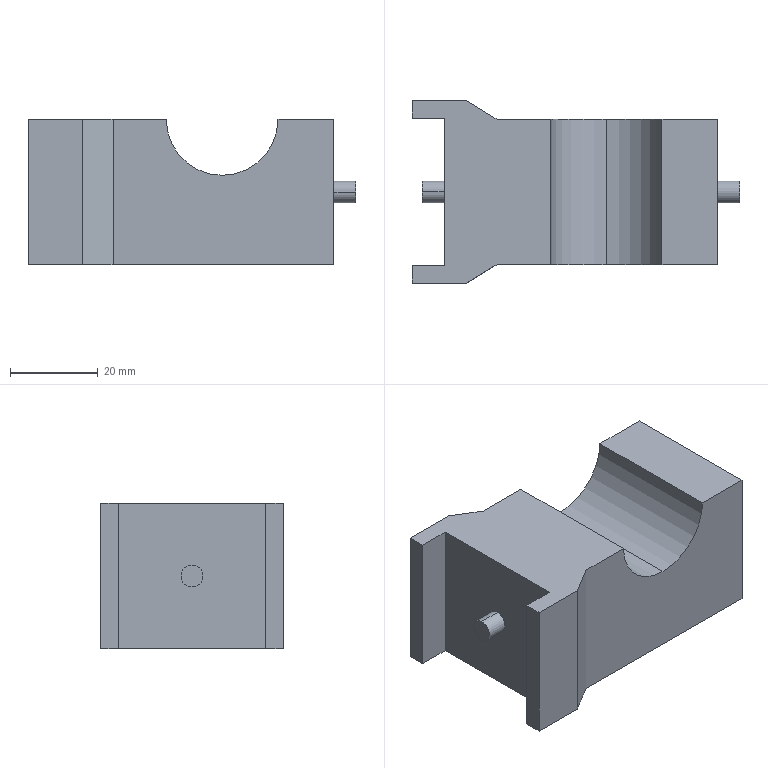Part | SolidWorks | features BaseBody 1, ICE 1 | 1 solid | 23 faces | box 74.5 x 41.5 x 33 mm | volume 63883 mm3 | plane 17 | cylinder 6 | commonest cylinder face diameters 5 x4 25.4 x2
STEP:
#1=CARTESIAN_POINT('',(12.4,16.5,16.5));
#2=VERTEX_POINT('',#1);
#3=CARTESIAN_POINT('',(-0.3,16.5,3.8));
#4=VERTEX_POINT('',#3);
#5=CARTESIAN_POINT('',(-0.3,16.5,16.5));
#6=DIRECTION('',(0.,1.,0.));
#7=DIRECTION('',(1.,0.,0.));
#8=AXIS2_PLACEMENT_3D('',#5,#6,#7);
#9=CIRCLE('',#8,12.7);
#10=EDGE_CURVE('',#2,#4,#9,.T.);
#11=ORIENTED_EDGE('',*,*,#10,.T.);
#12=CARTESIAN_POINT('',(-0.3,-16.5,3.8));
#13=VERTEX_POINT('',#12);
#14=CARTESIAN_POINT('',(-0.3,20.75,3.8));
#15=DIRECTION('',(0.,-1.,0.));
#16=VECTOR('',#15,1000.);
#17=LINE('',#14,#16);
#18=EDGE_CURVE('',#4,#13,#17,.T.);
#19=ORIENTED_EDGE('',*,*,#18,.T.);
#20=CARTESIAN_POINT('',(12.4,-16.5,16.5));
#21=VERTEX_POINT('',#20);
#22=CARTESIAN_POINT('',(-0.3,-16.5,16.5));
#23=DIRECTION('',(0.,-1.,0.));
#24=DIRECTION('',(0.,0.,1.));
#25=AXIS2_PLACEMENT_3D('',#22,#23,#24);
#26=CIRCLE('',#25,12.7);
#27=EDGE_CURVE('',#13,#21,#26,.T.);
#28=ORIENTED_EDGE('',*,*,#27,.T.);
#29=CARTESIAN_POINT('',(12.4,20.75,16.5));
#30=DIRECTION('',(0.,1.,0.));
#31=VECTOR('',#30,1000.);
#32=LINE('',#29,#31);
#33=EDGE_CURVE('',#21,#2,#32,.T.);
#34=ORIENTED_EDGE('',*,*,#33,.T.);
#35=EDGE_LOOP('',(#11,#19,#28,#34));
#36=FACE_OUTER_BOUND('',#35,.T.);
#37=CARTESIAN_POINT('',(-0.3,20.75,16.5));
#38=DIRECTION('',(0.,-1.,0.));
#39=DIRECTION('',(0.,0.,-1.));
#40=AXIS2_PLACEMENT_3D('',#37,#38,#39);
#41=CYLINDRICAL_SURFACE('',#40,12.7);
#42=ADVANCED_FACE('',(#36),#41,.F.);
#43=CARTESIAN_POINT('',(30.1,2.5,0.));
#44=VERTEX_POINT('',#43);
#45=CARTESIAN_POINT('',(30.1,-2.5,0.));
#46=VERTEX_POINT('',#45);
#47=CARTESIAN_POINT('',(30.1,0.,0.));
#48=DIRECTION('',(1.,0.,0.));
#49=DIRECTION('',(0.,1.,0.));
#50=AXIS2_PLACEMENT_3D('',#47,#48,#49);
#51=CIRCLE('',#50,2.5);
#52=EDGE_CURVE('',#44,#46,#51,.T.);
#53=ORIENTED_EDGE('',*,*,#52,.F.);
#54=CARTESIAN_POINT('',(25.1,2.5,0.));
#55=VERTEX_POINT('',#54);
#56=CARTESIAN_POINT('',(30.1,2.5,0.));
#57=DIRECTION('',(-1.,0.,0.));
#58=VECTOR('',#57,1000.);
#59=LINE('',#56,#58);
#60=EDGE_CURVE('',#44,#55,#59,.T.);
#61=ORIENTED_EDGE('',*,*,#60,.T.);
#62=CARTESIAN_POINT('',(25.1,-2.5,0.));
#63=VERTEX_POINT('',#62);
#64=CARTESIAN_POINT('',(25.1,0.,0.));
#65=DIRECTION('',(1.,0.,0.));
#66=DIRECTION('',(0.,-1.,0.));
#67=AXIS2_PLACEMENT_3D('',#64,#65,#66);
#68=CIRCLE('',#67,2.5);
#69=EDGE_CURVE('',#55,#63,#68,.T.);
#70=ORIENTED_EDGE('',*,*,#69,.T.);
#71=CARTESIAN_POINT('',(30.1,-2.5,0.));
#72=DIRECTION('',(-1.,0.,0.));
#73=VECTOR('',#72,1000.);
#74=LINE('',#71,#73);
#75=EDGE_CURVE('',#46,#63,#74,.T.);
#76=ORIENTED_EDGE('',*,*,#75,.F.);
#77=EDGE_LOOP('',(#53,#61,#70,#76));
#78=FACE_OUTER_BOUND('',#77,.T.);
#79=CARTESIAN_POINT('',(30.1,0.,0.));
#80=DIRECTION('',(-1.,0.,0.));
#81=DIRECTION('',(0.,-1.,0.));
#82=AXIS2_PLACEMENT_3D('',#79,#80,#81);
#83=CYLINDRICAL_SURFACE('',#82,2.5);
#84=ADVANCED_FACE('',(#78),#83,.T.);
#85=CARTESIAN_POINT('',(-42.1,0.,2.5));
#86=VERTEX_POINT('',#85);
#87=CARTESIAN_POINT('',(-42.1,0.,-2.5));
#88=VERTEX_POINT('',#87);
#89=CARTESIAN_POINT('',(-42.1,0.,0.));
#90=DIRECTION('',(-1.,0.,0.));
#91=DIRECTION('',(0.,0.,1.));
#92=AXIS2_PLACEMENT_3D('',#89,#90,#91);
#93=CIRCLE('',#92,2.5);
#94=EDGE_CURVE('',#86,#88,#93,.T.);
#95=ORIENTED_EDGE('',*,*,#94,.F.);
#96=CARTESIAN_POINT('',(-37.1,0.,2.5));
#97=VERTEX_POINT('',#96);
#98=CARTESIAN_POINT('',(-42.1,0.,2.5));
#99=DIRECTION('',(1.,0.,0.));
#100=VECTOR('',#99,1000.);
#101=LINE('',#98,#100);
#102=EDGE_CURVE('',#86,#97,#101,.T.);
#103=ORIENTED_EDGE('',*,*,#102,.T.);
#104=CARTESIAN_POINT('',(-37.1,0.,-2.5));
#105=VERTEX_POINT('',#104);
#106=CARTESIAN_POINT('',(-37.1,0.,0.));
#107=DIRECTION('',(-1.,0.,0.));
#108=DIRECTION('',(0.,1.,0.));
#109=AXIS2_PLACEMENT_3D('',#106,#107,#108);
#110=CIRCLE('',#109,2.5);
#111=EDGE_CURVE('',#97,#105,#110,.T.);
#112=ORIENTED_EDGE('',*,*,#111,.T.);
#113=CARTESIAN_POINT('',(-42.1,0.,-2.5));
#114=DIRECTION('',(1.,0.,0.));
#115=VECTOR('',#114,1000.);
#116=LINE('',#113,#115);
#117=EDGE_CURVE('',#88,#105,#116,.T.);
#118=ORIENTED_EDGE('',*,*,#117,.F.);
#119=EDGE_LOOP('',(#95,#103,#112,#118));
#120=FACE_OUTER_BOUND('',#119,.T.);
#121=CARTESIAN_POINT('',(-42.1,0.,0.));
#122=DIRECTION('',(1.,0.,0.));
#123=DIRECTION('',(0.,0.,-1.));
#124=AXIS2_PLACEMENT_3D('',#121,#122,#123);
#125=CYLINDRICAL_SURFACE('',#124,2.5);
#126=ADVANCED_FACE('',(#120),#125,.T.);
#127=ORIENTED_EDGE('',*,*,#33,.F.);
#128=CARTESIAN_POINT('',(25.1,-16.5,16.5));
#129=VERTEX_POINT('',#128);
#130=CARTESIAN_POINT('',(25.1,-16.5,16.5));
#131=DIRECTION('',(1.,0.,0.));
#132=VECTOR('',#131,1000.);
#133=LINE('',#130,#132);
#134=EDGE_CURVE('',#21,#129,#133,.T.);
#135=ORIENTED_EDGE('',*,*,#134,.T.);
#136=CARTESIAN_POINT('',(25.1,16.5,16.5));
#137=VERTEX_POINT('',#136);
#138=CARTESIAN_POINT('',(25.1,16.5,16.5));
#139=DIRECTION('',(0.,1.,0.));
#140=VECTOR('',#139,1000.);
#141=LINE('',#138,#140);
#142=EDGE_CURVE('',#129,#137,#141,.T.);
#143=ORIENTED_EDGE('',*,*,#142,.T.);
#144=CARTESIAN_POINT('',(25.1,16.5,16.5));
#145=DIRECTION('',(-1.,0.,0.));
#146=VECTOR('',#145,1000.);
#147=LINE('',#144,#146);
#148=EDGE_CURVE('',#137,#2,#147,.T.);
#149=ORIENTED_EDGE('',*,*,#148,.T.);
#150=EDGE_LOOP('',(#127,#135,#143,#149));
#151=FACE_OUTER_BOUND('',#150,.T.);
#152=CARTESIAN_POINT('',(0.,0.,16.5));
#153=DIRECTION('',(0.,0.,-1.));
#154=DIRECTION('',(-1.,0.,0.));
#155=AXIS2_PLACEMENT_3D('',#152,#153,#154);
#156=PLANE('',#155);
#157=ADVANCED_FACE('',(#151),#156,.F.);
#158=CARTESIAN_POINT('',(-13.,16.5,16.5));
#159=VERTEX_POINT('',#158);
#160=CARTESIAN_POINT('',(-13.,-16.5,16.5));
#161=VERTEX_POINT('',#160);
#162=CARTESIAN_POINT('',(-13.,20.75,16.5));
#163=DIRECTION('',(0.,-1.,0.));
#164=VECTOR('',#163,1000.);
#165=LINE('',#162,#164);
#166=EDGE_CURVE('',#159,#161,#165,.T.);
#167=ORIENTED_EDGE('',*,*,#166,.F.);
#168=CARTESIAN_POINT('',(-25.1,16.5,16.5));
#169=VERTEX_POINT('',#168);
#170=CARTESIAN_POINT('',(25.1,16.5,16.5));
#171=DIRECTION('',(-1.,0.,0.));
#172=VECTOR('',#171,1000.);
#173=LINE('',#170,#172);
#174=EDGE_CURVE('',#159,#169,#173,.T.);
#175=ORIENTED_EDGE('',*,*,#174,.T.);
#176=CARTESIAN_POINT('',(-32.1,20.75,16.5));
#177=VERTEX_POINT('',#176);
#178=CARTESIAN_POINT('',(-32.1,20.75,16.5));
#179=DIRECTION('',(-0.8548,0.519,0.));
#180=VECTOR('',#179,1000.);
#181=LINE('',#178,#180);
#182=EDGE_CURVE('',#169,#177,#181,.T.);
#183=ORIENTED_EDGE('',*,*,#182,.T.);
#184=CARTESIAN_POINT('',(-44.4,20.75,16.5));
#185=VERTEX_POINT('',#184);
#186=CARTESIAN_POINT('',(-44.4,20.75,16.5));
#187=DIRECTION('',(-1.,0.,0.));
#188=VECTOR('',#187,1000.);
#189=LINE('',#186,#188);
#190=EDGE_CURVE('',#177,#185,#189,.T.);
#191=ORIENTED_EDGE('',*,*,#190,.T.);
#192=CARTESIAN_POINT('',(-44.4,16.75,16.5));
#193=VERTEX_POINT('',#192);
#194=CARTESIAN_POINT('',(-44.4,20.75,16.5));
#195=DIRECTION('',(0.,-1.,0.));
#196=VECTOR('',#195,1000.);
#197=LINE('',#194,#196);
#198=EDGE_CURVE('',#185,#193,#197,.T.);
#199=ORIENTED_EDGE('',*,*,#198,.T.);
#200=CARTESIAN_POINT('',(-37.1,16.75,16.5));
#201=VERTEX_POINT('',#200);
#202=CARTESIAN_POINT('',(-44.4,16.75,16.5));
#203=DIRECTION('',(1.,0.,0.));
#204=VECTOR('',#203,1000.);
#205=LINE('',#202,#204);
#206=EDGE_CURVE('',#193,#201,#205,.T.);
#207=ORIENTED_EDGE('',*,*,#206,.T.);
#208=CARTESIAN_POINT('',(-37.1,-16.75,16.5));
#209=VERTEX_POINT('',#208);
#210=CARTESIAN_POINT('',(-37.1,16.75,16.5));
#211=DIRECTION('',(0.,-1.,0.));
#212=VECTOR('',#211,1000.);
#213=LINE('',#210,#212);
#214=EDGE_CURVE('',#201,#209,#213,.T.);
#215=ORIENTED_EDGE('',*,*,#214,.T.);
#216=CARTESIAN_POINT('',(-44.4,-16.75,16.5));
#217=VERTEX_POINT('',#216);
#218=CARTESIAN_POINT('',(-44.4,-16.75,16.5));
#219=DIRECTION('',(-1.,0.,0.));
#220=VECTOR('',#219,1000.);
#221=LINE('',#218,#220);
#222=EDGE_CURVE('',#209,#217,#221,.T.);
#223=ORIENTED_EDGE('',*,*,#222,.T.);
#224=CARTESIAN_POINT('',(-44.4,-20.75,16.5));
#225=VERTEX_POINT('',#224);
#226=CARTESIAN_POINT('',(-44.4,-20.75,16.5));
#227=DIRECTION('',(0.,-1.,0.));
#228=VECTOR('',#227,1000.);
#229=LINE('',#226,#228);
#230=EDGE_CURVE('',#217,#225,#229,.T.);
#231=ORIENTED_EDGE('',*,*,#230,.T.);
#232=CARTESIAN_POINT('',(-32.1,-20.75,16.5));
#233=VERTEX_POINT('',#232);
#234=CARTESIAN_POINT('',(-44.4,-20.75,16.5));
#235=DIRECTION('',(1.,0.,0.));
#236=VECTOR('',#235,1000.);
#237=LINE('',#234,#236);
#238=EDGE_CURVE('',#225,#233,#237,.T.);
#239=ORIENTED_EDGE('',*,*,#238,.T.);
#240=CARTESIAN_POINT('',(-25.1,-16.5,16.5));
#241=VERTEX_POINT('',#240);
#242=CARTESIAN_POINT('',(-32.1,-20.75,16.5));
#243=DIRECTION('',(0.8548,0.519,0.));
#244=VECTOR('',#243,1000.);
#245=LINE('',#242,#244);
#246=EDGE_CURVE('',#233,#241,#245,.T.);
#247=ORIENTED_EDGE('',*,*,#246,.T.);
#248=CARTESIAN_POINT('',(25.1,-16.5,16.5));
#249=DIRECTION('',(1.,0.,0.));
#250=VECTOR('',#249,1000.);
#251=LINE('',#248,#250);
#252=EDGE_CURVE('',#241,#161,#251,.T.);
#253=ORIENTED_EDGE('',*,*,#252,.T.);
#254=EDGE_LOOP('',(#167,#175,#183,#191,#199,#207,#215,#223,#231,#239,#247,#253));
#255=FACE_OUTER_BOUND('',#254,.T.);
#256=CARTESIAN_POINT('',(0.,0.,16.5));
#257=DIRECTION('',(0.,0.,-1.));
#258=DIRECTION('',(-1.,0.,0.));
#259=AXIS2_PLACEMENT_3D('',#256,#257,#258);
#260=PLANE('',#259);
#261=ADVANCED_FACE('',(#255),#260,.F.);
#262=CARTESIAN_POINT('',(25.1,-16.5,-16.5));
#263=VERTEX_POINT('',#262);
#264=CARTESIAN_POINT('',(25.1,16.5,-16.5));
#265=VERTEX_POINT('',#264);
#266=CARTESIAN_POINT('',(25.1,16.5,-16.5));
#267=DIRECTION('',(0.,1.,0.));
#268=VECTOR('',#267,1000.);
#269=LINE('',#266,#268);
#270=EDGE_CURVE('',#263,#265,#269,.T.);
#271=ORIENTED_EDGE('',*,*,#270,.T.);
#272=CARTESIAN_POINT('',(25.1,16.5,16.5));
#273=DIRECTION('',(0.,0.,-1.));
#274=VECTOR('',#273,1000.);
#275=LINE('',#272,#274);
#276=EDGE_CURVE('',#137,#265,#275,.T.);
#277=ORIENTED_EDGE('',*,*,#276,.F.);
#278=ORIENTED_EDGE('',*,*,#142,.F.);
#279=CARTESIAN_POINT('',(25.1,-16.5,16.5));
#280=DIRECTION('',(0.,0.,-1.));
#281=VECTOR('',#280,1000.);
#282=LINE('',#279,#281);
#283=EDGE_CURVE('',#129,#263,#282,.T.);
#284=ORIENTED_EDGE('',*,*,#283,.T.);
#285=EDGE_LOOP('',(#271,#277,#278,#284));
#286=FACE_OUTER_BOUND('',#285,.T.);
#287=CARTESIAN_POINT('',(25.1,0.,0.));
#288=DIRECTION('',(1.,0.,0.));
#289=DIRECTION('',(0.,-1.,0.));
#290=AXIS2_PLACEMENT_3D('',#287,#288,#289);
#291=CIRCLE('',#290,2.5);
#292=EDGE_CURVE('',#63,#55,#291,.T.);
#293=ORIENTED_EDGE('',*,*,#292,.F.);
#294=ORIENTED_EDGE('',*,*,#69,.F.);
#295=EDGE_LOOP('',(#293,#294));
#296=FACE_BOUND('',#295,.T.);
#297=CARTESIAN_POINT('',(25.1,16.5,16.5));
#298=DIRECTION('',(-1.,0.,0.));
#299=DIRECTION('',(0.,-1.,0.));
#300=AXIS2_PLACEMENT_3D('',#297,#298,#299);
#301=PLANE('',#300);
#302=ADVANCED_FACE('',(#286,#296),#301,.F.);
#303=CARTESIAN_POINT('',(-37.1,16.75,-16.5));
#304=VERTEX_POINT('',#303);
#305=CARTESIAN_POINT('',(-37.1,-16.75,-16.5));
#306=VERTEX_POINT('',#305);
#307=CARTESIAN_POINT('',(-37.1,16.75,-16.5));
#308=DIRECTION('',(0.,-1.,0.));
#309=VECTOR('',#308,1000.);
#310=LINE('',#307,#309);
#311=EDGE_CURVE('',#304,#306,#310,.T.);
#312=ORIENTED_EDGE('',*,*,#311,.T.);
#313=CARTESIAN_POINT('',(-37.1,-16.75,16.5));
#314=DIRECTION('',(0.,0.,-1.));
#315=VECTOR('',#314,1000.);
#316=LINE('',#313,#315);
#317=EDGE_CURVE('',#209,#306,#316,.T.);
#318=ORIENTED_EDGE('',*,*,#317,.F.);
#319=ORIENTED_EDGE('',*,*,#214,.F.);
#320=CARTESIAN_POINT('',(-37.1,16.75,16.5));
#321=DIRECTION('',(0.,0.,-1.));
#322=VECTOR('',#321,1000.);
#323=LINE('',#320,#322);
#324=EDGE_CURVE('',#201,#304,#323,.T.);
#325=ORIENTED_EDGE('',*,*,#324,.T.);
#326=EDGE_LOOP('',(#312,#318,#319,#325));
#327=FACE_OUTER_BOUND('',#326,.T.);
#328=CARTESIAN_POINT('',(-37.1,0.,0.));
#329=DIRECTION('',(-1.,0.,0.));
#330=DIRECTION('',(0.,1.,0.));
#331=AXIS2_PLACEMENT_3D('',#328,#329,#330);
#332=CIRCLE('',#331,2.5);
#333=EDGE_CURVE('',#105,#97,#332,.T.);
#334=ORIENTED_EDGE('',*,*,#333,.F.);
#335=ORIENTED_EDGE('',*,*,#111,.F.);
#336=EDGE_LOOP('',(#334,#335));
#337=FACE_BOUND('',#336,.T.);
#338=CARTESIAN_POINT('',(-37.1,16.75,16.5));
#339=DIRECTION('',(1.,0.,0.));
#340=DIRECTION('',(0.,1.,0.));
#341=AXIS2_PLACEMENT_3D('',#338,#339,#340);
#342=PLANE('',#341);
#343=ADVANCED_FACE('',(#327,#337),#342,.F.);
#344=ORIENTED_EDGE('',*,*,#10,.F.);
#345=ORIENTED_EDGE('',*,*,#148,.F.);
#346=ORIENTED_EDGE('',*,*,#276,.T.);
#347=CARTESIAN_POINT('',(-25.1,16.5,-16.5));
#348=VERTEX_POINT('',#347);
#349=CARTESIAN_POINT('',(25.1,16.5,-16.5));
#350=DIRECTION('',(-1.,0.,0.));
#351=VECTOR('',#350,1000.);
#352=LINE('',#349,#351);
#353=EDGE_CURVE('',#265,#348,#352,.T.);
#354=ORIENTED_EDGE('',*,*,#353,.T.);
#355=CARTESIAN_POINT('',(-25.1,16.5,16.5));
#356=DIRECTION('',(0.,0.,-1.));
#357=VECTOR('',#356,1000.);
#358=LINE('',#355,#357);
#359=EDGE_CURVE('',#169,#348,#358,.T.);
#360=ORIENTED_EDGE('',*,*,#359,.F.);
#361=ORIENTED_EDGE('',*,*,#174,.F.);
#362=CARTESIAN_POINT('',(-0.3,16.5,16.5));
#363=DIRECTION('',(0.,1.,0.));
#364=DIRECTION('',(1.,0.,0.));
#365=AXIS2_PLACEMENT_3D('',#362,#363,#364);
#366=CIRCLE('',#365,12.7);
#367=EDGE_CURVE('',#4,#159,#366,.T.);
#368=ORIENTED_EDGE('',*,*,#367,.F.);
#369=EDGE_LOOP('',(#344,#345,#346,#354,#360,#361,#368));
#370=FACE_OUTER_BOUND('',#369,.T.);
#371=CARTESIAN_POINT('',(25.1,16.5,16.5));
#372=DIRECTION('',(0.,-1.,0.));
#373=DIRECTION('',(1.,0.,0.));
#374=AXIS2_PLACEMENT_3D('',#371,#372,#373);
#375=PLANE('',#374);
#376=ADVANCED_FACE('',(#370),#375,.F.);
#377=CARTESIAN_POINT('',(-32.1,20.75,-16.5));
#378=VERTEX_POINT('',#377);
#379=CARTESIAN_POINT('',(-32.1,20.75,-16.5));
#380=DIRECTION('',(-0.8548,0.519,0.));
#381=VECTOR('',#380,1000.);
#382=LINE('',#379,#381);
#383=EDGE_CURVE('',#348,#378,#382,.T.);
#384=ORIENTED_EDGE('',*,*,#383,.T.);
#385=CARTESIAN_POINT('',(-32.1,20.75,16.5));
#386=DIRECTION('',(0.,0.,-1.));
#387=VECTOR('',#386,1000.);
#388=LINE('',#385,#387);
#389=EDGE_CURVE('',#177,#378,#388,.T.);
#390=ORIENTED_EDGE('',*,*,#389,.F.);
#391=ORIENTED_EDGE('',*,*,#182,.F.);
#392=ORIENTED_EDGE('',*,*,#359,.T.);
#393=EDGE_LOOP('',(#384,#390,#391,#392));
#394=FACE_OUTER_BOUND('',#393,.T.);
#395=CARTESIAN_POINT('',(-32.1,20.75,16.5));
#396=DIRECTION('',(-0.519,-0.8548,0.));
#397=DIRECTION('',(0.8548,-0.519,0.));
#398=AXIS2_PLACEMENT_3D('',#395,#396,#397);
#399=PLANE('',#398);
#400=ADVANCED_FACE('',(#394),#399,.F.);
#401=CARTESIAN_POINT('',(-44.4,20.75,-16.5));
#402=VERTEX_POINT('',#401);
#403=CARTESIAN_POINT('',(-44.4,20.75,-16.5));
#404=DIRECTION('',(-1.,0.,0.));
#405=VECTOR('',#404,1000.);
#406=LINE('',#403,#405);
#407=EDGE_CURVE('',#378,#402,#406,.T.);
#408=ORIENTED_EDGE('',*,*,#407,.T.);
#409=CARTESIAN_POINT('',(-44.4,20.75,16.5));
#410=DIRECTION('',(0.,0.,-1.));
#411=VECTOR('',#410,1000.);
#412=LINE('',#409,#411);
#413=EDGE_CURVE('',#185,#402,#412,.T.);
#414=ORIENTED_EDGE('',*,*,#413,.F.);
#415=ORIENTED_EDGE('',*,*,#190,.F.);
#416=ORIENTED_EDGE('',*,*,#389,.T.);
#417=EDGE_LOOP('',(#408,#414,#415,#416));
#418=FACE_OUTER_BOUND('',#417,.T.);
#419=CARTESIAN_POINT('',(-44.4,20.75,16.5));
#420=DIRECTION('',(0.,-1.,0.));
#421=DIRECTION('',(1.,0.,0.));
#422=AXIS2_PLACEMENT_3D('',#419,#420,#421);
#423=PLANE('',#422);
#424=ADVANCED_FACE('',(#418),#423,.F.);
#425=CARTESIAN_POINT('',(-44.4,16.75,-16.5));
#426=VERTEX_POINT('',#425);
#427=CARTESIAN_POINT('',(-44.4,20.75,-16.5));
#428=DIRECTION('',(0.,-1.,0.));
#429=VECTOR('',#428,1000.);
#430=LINE('',#427,#429);
#431=EDGE_CURVE('',#402,#426,#430,.T.);
#432=ORIENTED_EDGE('',*,*,#431,.T.);
#433=CARTESIAN_POINT('',(-44.4,16.75,16.5));
#434=DIRECTION('',(0.,0.,-1.));
#435=VECTOR('',#434,1000.);
#436=LINE('',#433,#435);
#437=EDGE_CURVE('',#193,#426,#436,.T.);
#438=ORIENTED_EDGE('',*,*,#437,.F.);
#439=ORIENTED_EDGE('',*,*,#198,.F.);
#440=ORIENTED_EDGE('',*,*,#413,.T.);
#441=EDGE_LOOP('',(#432,#438,#439,#440));
#442=FACE_OUTER_BOUND('',#441,.T.);
#443=CARTESIAN_POINT('',(-44.4,20.75,16.5));
#444=DIRECTION('',(1.,0.,0.));
#445=DIRECTION('',(0.,1.,0.));
#446=AXIS2_PLACEMENT_3D('',#443,#444,#445);
#447=PLANE('',#446);
#448=ADVANCED_FACE('',(#442),#447,.F.);
#449=CARTESIAN_POINT('',(-44.4,16.75,-16.5));
#450=DIRECTION('',(1.,0.,0.));
#451=VECTOR('',#450,1000.);
#452=LINE('',#449,#451);
#453=EDGE_CURVE('',#426,#304,#452,.T.);
#454=ORIENTED_EDGE('',*,*,#453,.T.);
#455=ORIENTED_EDGE('',*,*,#324,.F.);
#456=ORIENTED_EDGE('',*,*,#206,.F.);
#457=ORIENTED_EDGE('',*,*,#437,.T.);
#458=EDGE_LOOP('',(#454,#455,#456,#457));
#459=FACE_OUTER_BOUND('',#458,.T.);
#460=CARTESIAN_POINT('',(-44.4,16.75,16.5));
#461=DIRECTION('',(0.,1.,0.));
#462=DIRECTION('',(-1.,0.,0.));
#463=AXIS2_PLACEMENT_3D('',#460,#461,#462);
#464=PLANE('',#463);
#465=ADVANCED_FACE('',(#459),#464,.F.);
#466=CARTESIAN_POINT('',(-44.4,-16.75,-16.5));
#467=VERTEX_POINT('',#466);
#468=CARTESIAN_POINT('',(-44.4,-16.75,-16.5));
#469=DIRECTION('',(-1.,0.,0.));
#470=VECTOR('',#469,1000.);
#471=LINE('',#468,#470);
#472=EDGE_CURVE('',#306,#467,#471,.T.);
#473=ORIENTED_EDGE('',*,*,#472,.T.);
#474=CARTESIAN_POINT('',(-44.4,-16.75,16.5));
#475=DIRECTION('',(0.,0.,-1.));
#476=VECTOR('',#475,1000.);
#477=LINE('',#474,#476);
#478=EDGE_CURVE('',#217,#467,#477,.T.);
#479=ORIENTED_EDGE('',*,*,#478,.F.);
#480=ORIENTED_EDGE('',*,*,#222,.F.);
#481=ORIENTED_EDGE('',*,*,#317,.T.);
#482=EDGE_LOOP('',(#473,#479,#480,#481));
#483=FACE_OUTER_BOUND('',#482,.T.);
#484=CARTESIAN_POINT('',(-44.4,-16.75,16.5));
#485=DIRECTION('',(0.,-1.,0.));
#486=DIRECTION('',(1.,0.,0.));
#487=AXIS2_PLACEMENT_3D('',#484,#485,#486);
#488=PLANE('',#487);
#489=ADVANCED_FACE('',(#483),#488,.F.);
#490=CARTESIAN_POINT('',(-44.4,-20.75,-16.5));
#491=VERTEX_POINT('',#490);
#492=CARTESIAN_POINT('',(-44.4,-20.75,-16.5));
#493=DIRECTION('',(0.,-1.,0.));
#494=VECTOR('',#493,1000.);
#495=LINE('',#492,#494);
#496=EDGE_CURVE('',#467,#491,#495,.T.);
#497=ORIENTED_EDGE('',*,*,#496,.T.);
#498=CARTESIAN_POINT('',(-44.4,-20.75,16.5));
#499=DIRECTION('',(0.,0.,-1.));
#500=VECTOR('',#499,1000.);
#501=LINE('',#498,#500);
#502=EDGE_CURVE('',#225,#491,#501,.T.);
#503=ORIENTED_EDGE('',*,*,#502,.F.);
#504=ORIENTED_EDGE('',*,*,#230,.F.);
#505=ORIENTED_EDGE('',*,*,#478,.T.);
#506=EDGE_LOOP('',(#497,#503,#504,#505));
#507=FACE_OUTER_BOUND('',#506,.T.);
#508=CARTESIAN_POINT('',(-44.4,-20.75,16.5));
#509=DIRECTION('',(1.,0.,0.));
#510=DIRECTION('',(0.,1.,0.));
#511=AXIS2_PLACEMENT_3D('',#508,#509,#510);
#512=PLANE('',#511);
#513=ADVANCED_FACE('',(#507),#512,.F.);
#514=CARTESIAN_POINT('',(-32.1,-20.75,-16.5));
#515=VERTEX_POINT('',#514);
#516=CARTESIAN_POINT('',(-44.4,-20.75,-16.5));
#517=DIRECTION('',(1.,0.,0.));
#518=VECTOR('',#517,1000.);
#519=LINE('',#516,#518);
#520=EDGE_CURVE('',#491,#515,#519,.T.);
#521=ORIENTED_EDGE('',*,*,#520,.T.);
#522=CARTESIAN_POINT('',(-32.1,-20.75,16.5));
#523=DIRECTION('',(0.,0.,-1.));
#524=VECTOR('',#523,1000.);
#525=LINE('',#522,#524);
#526=EDGE_CURVE('',#233,#515,#525,.T.);
#527=ORIENTED_EDGE('',*,*,#526,.F.);
#528=ORIENTED_EDGE('',*,*,#238,.F.);
#529=ORIENTED_EDGE('',*,*,#502,.T.);
#530=EDGE_LOOP('',(#521,#527,#528,#529));
#531=FACE_OUTER_BOUND('',#530,.T.);
#532=CARTESIAN_POINT('',(-44.4,-20.75,16.5));
#533=DIRECTION('',(0.,1.,0.));
#534=DIRECTION('',(-1.,0.,0.));
#535=AXIS2_PLACEMENT_3D('',#532,#533,#534);
#536=PLANE('',#535);
#537=ADVANCED_FACE('',(#531),#536,.F.);
#538=CARTESIAN_POINT('',(-25.1,-16.5,-16.5));
#539=VERTEX_POINT('',#538);
#540=CARTESIAN_POINT('',(-32.1,-20.75,-16.5));
#541=DIRECTION('',(0.8548,0.519,0.));
#542=VECTOR('',#541,1000.);
#543=LINE('',#540,#542);
#544=EDGE_CURVE('',#515,#539,#543,.T.);
#545=ORIENTED_EDGE('',*,*,#544,.T.);
#546=CARTESIAN_POINT('',(-25.1,-16.5,16.5));
#547=DIRECTION('',(0.,0.,-1.));
#548=VECTOR('',#547,1000.);
#549=LINE('',#546,#548);
#550=EDGE_CURVE('',#241,#539,#549,.T.);
#551=ORIENTED_EDGE('',*,*,#550,.F.);
#552=ORIENTED_EDGE('',*,*,#246,.F.);
#553=ORIENTED_EDGE('',*,*,#526,.T.);
#554=EDGE_LOOP('',(#545,#551,#552,#553));
#555=FACE_OUTER_BOUND('',#554,.T.);
#556=CARTESIAN_POINT('',(-32.1,-20.75,16.5));
#557=DIRECTION('',(-0.519,0.8548,0.));
#558=DIRECTION('',(-0.8548,-0.519,0.));
#559=AXIS2_PLACEMENT_3D('',#556,#557,#558);
#560=PLANE('',#559);
#561=ADVANCED_FACE('',(#555),#560,.F.);
#562=CARTESIAN_POINT('',(-0.3,-16.5,16.5));
#563=DIRECTION('',(0.,-1.,0.));
#564=DIRECTION('',(0.,0.,1.));
#565=AXIS2_PLACEMENT_3D('',#562,#563,#564);
#566=CIRCLE('',#565,12.7);
#567=EDGE_CURVE('',#161,#13,#566,.T.);
#568=ORIENTED_EDGE('',*,*,#567,.F.);
#569=ORIENTED_EDGE('',*,*,#252,.F.);
#570=ORIENTED_EDGE('',*,*,#550,.T.);
#571=CARTESIAN_POINT('',(25.1,-16.5,-16.5));
#572=DIRECTION('',(1.,0.,0.));
#573=VECTOR('',#572,1000.);
#574=LINE('',#571,#573);
#575=EDGE_CURVE('',#539,#263,#574,.T.);
#576=ORIENTED_EDGE('',*,*,#575,.T.);
#577=ORIENTED_EDGE('',*,*,#283,.F.);
#578=ORIENTED_EDGE('',*,*,#134,.F.);
#579=ORIENTED_EDGE('',*,*,#27,.F.);
#580=EDGE_LOOP('',(#568,#569,#570,#576,#577,#578,#579));
#581=FACE_OUTER_BOUND('',#580,.T.);
#582=CARTESIAN_POINT('',(25.1,-16.5,16.5));
#583=DIRECTION('',(0.,1.,0.));
#584=DIRECTION('',(0.,0.,1.));
#585=AXIS2_PLACEMENT_3D('',#582,#583,#584);
#586=PLANE('',#585);
#587=ADVANCED_FACE('',(#581),#586,.F.);
#588=ORIENTED_EDGE('',*,*,#270,.F.);
#589=ORIENTED_EDGE('',*,*,#575,.F.);
#590=ORIENTED_EDGE('',*,*,#544,.F.);
#591=ORIENTED_EDGE('',*,*,#520,.F.);
#592=ORIENTED_EDGE('',*,*,#496,.F.);
#593=ORIENTED_EDGE('',*,*,#472,.F.);
#594=ORIENTED_EDGE('',*,*,#311,.F.);
#595=ORIENTED_EDGE('',*,*,#453,.F.);
#596=ORIENTED_EDGE('',*,*,#431,.F.);
#597=ORIENTED_EDGE('',*,*,#407,.F.);
#598=ORIENTED_EDGE('',*,*,#383,.F.);
#599=ORIENTED_EDGE('',*,*,#353,.F.);
#600=EDGE_LOOP('',(#588,#589,#590,#591,#592,#593,#594,#595,#596,#597,#598,#599));
#601=FACE_OUTER_BOUND('',#600,.T.);
#602=CARTESIAN_POINT('',(0.,0.,-16.5));
#603=DIRECTION('',(0.,0.,-1.));
#604=DIRECTION('',(-1.,0.,0.));
#605=AXIS2_PLACEMENT_3D('',#602,#603,#604);
#606=PLANE('',#605);
#607=ADVANCED_FACE('',(#601),#606,.T.);
#608=ORIENTED_EDGE('',*,*,#102,.F.);
#609=CARTESIAN_POINT('',(-42.1,0.,0.));
#610=DIRECTION('',(-1.,0.,0.));
#611=DIRECTION('',(0.,0.,1.));
#612=AXIS2_PLACEMENT_3D('',#609,#610,#611);
#613=CIRCLE('',#612,2.5);
#614=EDGE_CURVE('',#88,#86,#613,.T.);
#615=ORIENTED_EDGE('',*,*,#614,.F.);
#616=ORIENTED_EDGE('',*,*,#117,.T.);
#617=ORIENTED_EDGE('',*,*,#333,.T.);
#618=EDGE_LOOP('',(#608,#615,#616,#617));
#619=FACE_OUTER_BOUND('',#618,.T.);
#620=CARTESIAN_POINT('',(-42.1,0.,0.));
#621=DIRECTION('',(1.,0.,0.));
#622=DIRECTION('',(0.,0.,-1.));
#623=AXIS2_PLACEMENT_3D('',#620,#621,#622);
#624=CYLINDRICAL_SURFACE('',#623,2.5);
#625=ADVANCED_FACE('',(#619),#624,.T.);
#626=ORIENTED_EDGE('',*,*,#614,.T.);
#627=ORIENTED_EDGE('',*,*,#94,.T.);
#628=EDGE_LOOP('',(#626,#627));
#629=FACE_OUTER_BOUND('',#628,.T.);
#630=CARTESIAN_POINT('',(-42.1,0.,0.));
#631=DIRECTION('',(-1.,0.,0.));
#632=DIRECTION('',(0.,0.,1.));
#633=AXIS2_PLACEMENT_3D('',#630,#631,#632);
#634=PLANE('',#633);
#635=ADVANCED_FACE('',(#629),#634,.T.);
#636=ORIENTED_EDGE('',*,*,#60,.F.);
#637=CARTESIAN_POINT('',(30.1,0.,0.));
#638=DIRECTION('',(1.,0.,0.));
#639=DIRECTION('',(0.,1.,0.));
#640=AXIS2_PLACEMENT_3D('',#637,#638,#639);
#641=CIRCLE('',#640,2.5);
#642=EDGE_CURVE('',#46,#44,#641,.T.);
#643=ORIENTED_EDGE('',*,*,#642,.F.);
#644=ORIENTED_EDGE('',*,*,#75,.T.);
#645=ORIENTED_EDGE('',*,*,#292,.T.);
#646=EDGE_LOOP('',(#636,#643,#644,#645));
#647=FACE_OUTER_BOUND('',#646,.T.);
#648=CARTESIAN_POINT('',(30.1,0.,0.));
#649=DIRECTION('',(-1.,0.,0.));
#650=DIRECTION('',(0.,-1.,0.));
#651=AXIS2_PLACEMENT_3D('',#648,#649,#650);
#652=CYLINDRICAL_SURFACE('',#651,2.5);
#653=ADVANCED_FACE('',(#647),#652,.T.);
#654=ORIENTED_EDGE('',*,*,#642,.T.);
#655=ORIENTED_EDGE('',*,*,#52,.T.);
#656=EDGE_LOOP('',(#654,#655));
#657=FACE_OUTER_BOUND('',#656,.T.);
#658=CARTESIAN_POINT('',(30.1,0.,0.));
#659=DIRECTION('',(1.,0.,0.));
#660=DIRECTION('',(0.,1.,0.));
#661=AXIS2_PLACEMENT_3D('',#658,#659,#660);
#662=PLANE('',#661);
#663=ADVANCED_FACE('',(#657),#662,.T.);
#664=ORIENTED_EDGE('',*,*,#18,.F.);
#665=ORIENTED_EDGE('',*,*,#367,.T.);
#666=ORIENTED_EDGE('',*,*,#166,.T.);
#667=ORIENTED_EDGE('',*,*,#567,.T.);
#668=EDGE_LOOP('',(#664,#665,#666,#667));
#669=FACE_OUTER_BOUND('',#668,.T.);
#670=CARTESIAN_POINT('',(-0.3,20.75,16.5));
#671=DIRECTION('',(0.,-1.,0.));
#672=DIRECTION('',(0.,0.,-1.));
#673=AXIS2_PLACEMENT_3D('',#670,#671,#672);
#674=CYLINDRICAL_SURFACE('',#673,12.7);
#675=ADVANCED_FACE('',(#669),#674,.F.);
#676=CLOSED_SHELL('',(#42,#84,#126,#157,#261,#302,#343,#376,#400,#424,#448,#465,#489,#513,#537,#561,#587,#607,#625,#635,#653,#663,#675));
#677=MANIFOLD_SOLID_BREP('',#676);
#678=CARTESIAN_POINT('',(0.,0.,0.));
#679=DIRECTION('',(0.,0.,1.));
#680=DIRECTION('',(1.,0.,0.));
#681=AXIS2_PLACEMENT_3D('',#678,#679,#680);
#682=(LENGTH_UNIT()NAMED_UNIT(*)SI_UNIT(.MILLI.,.METRE.));
#683=UNCERTAINTY_MEASURE_WITH_UNIT(LENGTH_MEASURE(0.00001),#682,'','');
#684=(NAMED_UNIT(*)PLANE_ANGLE_UNIT()SI_UNIT($,.RADIAN.));
#685=(NAMED_UNIT(*)SI_UNIT($,.STERADIAN.)SOLID_ANGLE_UNIT());
#686=(GEOMETRIC_REPRESENTATION_CONTEXT(3)GLOBAL_UNCERTAINTY_ASSIGNED_CONTEXT((#683))GLOBAL_UNIT_ASSIGNED_CONTEXT((#682,#684,#685))REPRESENTATION_CONTEXT('',''));
#687=ADVANCED_BREP_SHAPE_REPRESENTATION('',(#677,#681),#686);